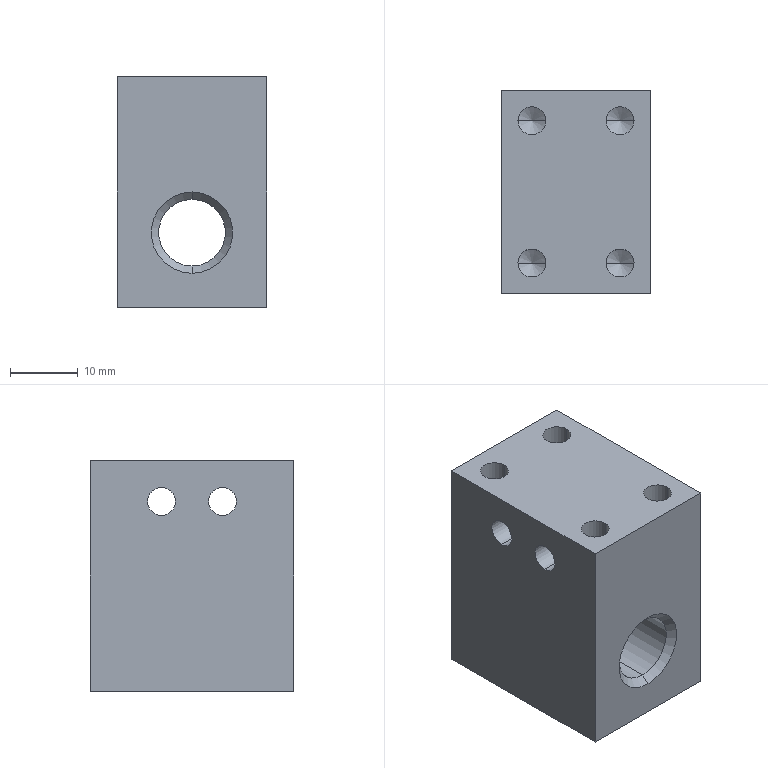Part | SolidWorks | features BaseBody 1 | 1 solid | 32 faces | box 22 x 30 x 34 mm | volume 18865 mm3 | cylinder 14 | cone 12 | plane 6 | commonest cylinder face diameters 4.134 x12 9.835 x2
STEP:
#1=CARTESIAN_POINT('',(279.547,1588.309,-1159.503));
#2=VERTEX_POINT('',#1);
#3=CARTESIAN_POINT('',(279.547,1588.309,-1163.637));
#4=VERTEX_POINT('',#3);
#5=CARTESIAN_POINT('',(279.547,1588.309,-1161.57));
#6=DIRECTION('',(1.,0.,0.));
#7=DIRECTION('',(0.,0.,-1.));
#8=AXIS2_PLACEMENT_3D('',#5,#6,#7);
#9=CIRCLE('',#8,2.067);
#10=EDGE_CURVE('',#2,#4,#9,.T.);
#11=ORIENTED_EDGE('',*,*,#10,.F.);
#12=CARTESIAN_POINT('',(301.547,1588.309,-1159.503));
#13=VERTEX_POINT('',#12);
#14=CARTESIAN_POINT('',(301.547,1588.309,-1159.503));
#15=DIRECTION('',(1.,0.,0.));
#16=VECTOR('',#15,1000.);
#17=LINE('',#14,#16);
#18=EDGE_CURVE('',#2,#13,#17,.T.);
#19=ORIENTED_EDGE('',*,*,#18,.T.);
#20=CARTESIAN_POINT('',(301.547,1588.309,-1163.637));
#21=VERTEX_POINT('',#20);
#22=CARTESIAN_POINT('',(301.547,1588.309,-1161.57));
#23=DIRECTION('',(1.,0.,0.));
#24=DIRECTION('',(0.,0.,-1.));
#25=AXIS2_PLACEMENT_3D('',#22,#23,#24);
#26=CIRCLE('',#25,2.067);
#27=EDGE_CURVE('',#13,#21,#26,.T.);
#28=ORIENTED_EDGE('',*,*,#27,.T.);
#29=CARTESIAN_POINT('',(301.547,1588.309,-1163.637));
#30=DIRECTION('',(1.,0.,0.));
#31=VECTOR('',#30,1000.);
#32=LINE('',#29,#31);
#33=EDGE_CURVE('',#4,#21,#32,.T.);
#34=ORIENTED_EDGE('',*,*,#33,.F.);
#35=EDGE_LOOP('',(#11,#19,#28,#34));
#36=FACE_OUTER_BOUND('',#35,.T.);
#37=CARTESIAN_POINT('',(301.547,1588.309,-1161.57));
#38=DIRECTION('',(1.,0.,0.));
#39=DIRECTION('',(0.,0.,-1.));
#40=AXIS2_PLACEMENT_3D('',#37,#38,#39);
#41=CYLINDRICAL_SURFACE('',#40,2.067);
#42=ADVANCED_FACE('',(#36),#41,.F.);
#43=CARTESIAN_POINT('',(279.547,1597.309,-1159.503));
#44=VERTEX_POINT('',#43);
#45=CARTESIAN_POINT('',(279.547,1597.309,-1163.637));
#46=VERTEX_POINT('',#45);
#47=CARTESIAN_POINT('',(279.547,1597.309,-1161.57));
#48=DIRECTION('',(1.,0.,0.));
#49=DIRECTION('',(0.,0.,-1.));
#50=AXIS2_PLACEMENT_3D('',#47,#48,#49);
#51=CIRCLE('',#50,2.067);
#52=EDGE_CURVE('',#44,#46,#51,.T.);
#53=ORIENTED_EDGE('',*,*,#52,.F.);
#54=CARTESIAN_POINT('',(301.547,1597.309,-1159.503));
#55=VERTEX_POINT('',#54);
#56=CARTESIAN_POINT('',(301.547,1597.309,-1159.503));
#57=DIRECTION('',(1.,0.,0.));
#58=VECTOR('',#57,1000.);
#59=LINE('',#56,#58);
#60=EDGE_CURVE('',#44,#55,#59,.T.);
#61=ORIENTED_EDGE('',*,*,#60,.T.);
#62=CARTESIAN_POINT('',(301.547,1597.309,-1163.637));
#63=VERTEX_POINT('',#62);
#64=CARTESIAN_POINT('',(301.547,1597.309,-1161.57));
#65=DIRECTION('',(1.,0.,0.));
#66=DIRECTION('',(0.,0.,-1.));
#67=AXIS2_PLACEMENT_3D('',#64,#65,#66);
#68=CIRCLE('',#67,2.067);
#69=EDGE_CURVE('',#55,#63,#68,.T.);
#70=ORIENTED_EDGE('',*,*,#69,.T.);
#71=CARTESIAN_POINT('',(301.547,1597.309,-1163.637));
#72=DIRECTION('',(1.,0.,0.));
#73=VECTOR('',#72,1000.);
#74=LINE('',#71,#73);
#75=EDGE_CURVE('',#46,#63,#74,.T.);
#76=ORIENTED_EDGE('',*,*,#75,.F.);
#77=EDGE_LOOP('',(#53,#61,#70,#76));
#78=FACE_OUTER_BOUND('',#77,.T.);
#79=CARTESIAN_POINT('',(301.547,1597.309,-1161.57));
#80=DIRECTION('',(1.,0.,0.));
#81=DIRECTION('',(0.,0.,-1.));
#82=AXIS2_PLACEMENT_3D('',#79,#80,#81);
#83=CYLINDRICAL_SURFACE('',#82,2.067);
#84=ADVANCED_FACE('',(#78),#83,.F.);
#85=CARTESIAN_POINT('',(290.547,1606.726,-1183.488));
#86=VERTEX_POINT('',#85);
#87=CARTESIAN_POINT('',(290.547,1606.726,-1173.652));
#88=VERTEX_POINT('',#87);
#89=CARTESIAN_POINT('',(290.547,1606.726,-1178.57));
#90=DIRECTION('',(0.,1.,0.));
#91=DIRECTION('',(-1.,0.,0.));
#92=AXIS2_PLACEMENT_3D('',#89,#90,#91);
#93=CIRCLE('',#92,4.918);
#94=EDGE_CURVE('',#86,#88,#93,.T.);
#95=ORIENTED_EDGE('',*,*,#94,.F.);
#96=CARTESIAN_POINT('',(290.547,1607.809,-1184.57));
#97=VERTEX_POINT('',#96);
#98=CARTESIAN_POINT('',(290.547,1607.809,-1184.57));
#99=DIRECTION('',(0.,0.7071,-0.7071));
#100=VECTOR('',#99,1000.);
#101=LINE('',#98,#100);
#102=EDGE_CURVE('',#86,#97,#101,.T.);
#103=ORIENTED_EDGE('',*,*,#102,.T.);
#104=CARTESIAN_POINT('',(290.547,1607.809,-1172.57));
#105=VERTEX_POINT('',#104);
#106=CARTESIAN_POINT('',(290.547,1607.809,-1178.57));
#107=DIRECTION('',(0.,-1.,0.));
#108=DIRECTION('',(0.,0.,1.));
#109=AXIS2_PLACEMENT_3D('',#106,#107,#108);
#110=CIRCLE('',#109,6.);
#111=EDGE_CURVE('',#105,#97,#110,.T.);
#112=ORIENTED_EDGE('',*,*,#111,.F.);
#113=CARTESIAN_POINT('',(290.547,1607.809,-1172.57));
#114=DIRECTION('',(0.,0.7071,0.7071));
#115=VECTOR('',#114,1000.);
#116=LINE('',#113,#115);
#117=EDGE_CURVE('',#88,#105,#116,.T.);
#118=ORIENTED_EDGE('',*,*,#117,.F.);
#119=EDGE_LOOP('',(#95,#103,#112,#118));
#120=FACE_OUTER_BOUND('',#119,.T.);
#121=CARTESIAN_POINT('',(290.547,1607.809,-1178.57));
#122=DIRECTION('',(0.,1.,0.));
#123=DIRECTION('',(0.,0.,1.));
#124=AXIS2_PLACEMENT_3D('',#121,#122,#123);
#125=CONICAL_SURFACE('',#124,6.,0.7854);
#126=ADVANCED_FACE('',(#120),#125,.F.);
#127=CARTESIAN_POINT('',(281.98,1603.309,-1167.57));
#128=VERTEX_POINT('',#127);
#129=CARTESIAN_POINT('',(286.114,1603.309,-1167.57));
#130=VERTEX_POINT('',#129);
#131=CARTESIAN_POINT('',(284.047,1603.309,-1167.57));
#132=DIRECTION('',(0.,0.,1.));
#133=DIRECTION('',(1.,0.,0.));
#134=AXIS2_PLACEMENT_3D('',#131,#132,#133);
#135=CIRCLE('',#134,2.067);
#136=EDGE_CURVE('',#128,#130,#135,.T.);
#137=ORIENTED_EDGE('',*,*,#136,.F.);
#138=CARTESIAN_POINT('',(281.98,1603.309,-1155.57));
#139=VERTEX_POINT('',#138);
#140=CARTESIAN_POINT('',(281.98,1603.309,-1155.57));
#141=DIRECTION('',(0.,0.,1.));
#142=VECTOR('',#141,1000.);
#143=LINE('',#140,#142);
#144=EDGE_CURVE('',#128,#139,#143,.T.);
#145=ORIENTED_EDGE('',*,*,#144,.T.);
#146=CARTESIAN_POINT('',(286.114,1603.309,-1155.57));
#147=VERTEX_POINT('',#146);
#148=CARTESIAN_POINT('',(284.047,1603.309,-1155.57));
#149=DIRECTION('',(0.,0.,1.));
#150=DIRECTION('',(1.,0.,0.));
#151=AXIS2_PLACEMENT_3D('',#148,#149,#150);
#152=CIRCLE('',#151,2.067);
#153=EDGE_CURVE('',#139,#147,#152,.T.);
#154=ORIENTED_EDGE('',*,*,#153,.T.);
#155=CARTESIAN_POINT('',(286.114,1603.309,-1155.57));
#156=DIRECTION('',(0.,0.,1.));
#157=VECTOR('',#156,1000.);
#158=LINE('',#155,#157);
#159=EDGE_CURVE('',#130,#147,#158,.T.);
#160=ORIENTED_EDGE('',*,*,#159,.F.);
#161=EDGE_LOOP('',(#137,#145,#154,#160));
#162=FACE_OUTER_BOUND('',#161,.T.);
#163=CARTESIAN_POINT('',(284.047,1603.309,-1155.57));
#164=DIRECTION('',(0.,0.,1.));
#165=DIRECTION('',(1.,0.,0.));
#166=AXIS2_PLACEMENT_3D('',#163,#164,#165);
#167=CYLINDRICAL_SURFACE('',#166,2.067);
#168=ADVANCED_FACE('',(#162),#167,.F.);
#169=CARTESIAN_POINT('',(294.98,1603.309,-1167.57));
#170=VERTEX_POINT('',#169);
#171=CARTESIAN_POINT('',(299.114,1603.309,-1167.57));
#172=VERTEX_POINT('',#171);
#173=CARTESIAN_POINT('',(297.047,1603.309,-1167.57));
#174=DIRECTION('',(0.,0.,1.));
#175=DIRECTION('',(1.,0.,0.));
#176=AXIS2_PLACEMENT_3D('',#173,#174,#175);
#177=CIRCLE('',#176,2.067);
#178=EDGE_CURVE('',#170,#172,#177,.T.);
#179=ORIENTED_EDGE('',*,*,#178,.F.);
#180=CARTESIAN_POINT('',(294.98,1603.309,-1155.57));
#181=VERTEX_POINT('',#180);
#182=CARTESIAN_POINT('',(294.98,1603.309,-1155.57));
#183=DIRECTION('',(0.,0.,1.));
#184=VECTOR('',#183,1000.);
#185=LINE('',#182,#184);
#186=EDGE_CURVE('',#170,#181,#185,.T.);
#187=ORIENTED_EDGE('',*,*,#186,.T.);
#188=CARTESIAN_POINT('',(299.114,1603.309,-1155.57));
#189=VERTEX_POINT('',#188);
#190=CARTESIAN_POINT('',(297.047,1603.309,-1155.57));
#191=DIRECTION('',(0.,0.,1.));
#192=DIRECTION('',(1.,0.,0.));
#193=AXIS2_PLACEMENT_3D('',#190,#191,#192);
#194=CIRCLE('',#193,2.067);
#195=EDGE_CURVE('',#181,#189,#194,.T.);
#196=ORIENTED_EDGE('',*,*,#195,.T.);
#197=CARTESIAN_POINT('',(299.114,1603.309,-1155.57));
#198=DIRECTION('',(0.,0.,1.));
#199=VECTOR('',#198,1000.);
#200=LINE('',#197,#199);
#201=EDGE_CURVE('',#172,#189,#200,.T.);
#202=ORIENTED_EDGE('',*,*,#201,.F.);
#203=EDGE_LOOP('',(#179,#187,#196,#202));
#204=FACE_OUTER_BOUND('',#203,.T.);
#205=CARTESIAN_POINT('',(297.047,1603.309,-1155.57));
#206=DIRECTION('',(0.,0.,1.));
#207=DIRECTION('',(1.,0.,0.));
#208=AXIS2_PLACEMENT_3D('',#205,#206,#207);
#209=CYLINDRICAL_SURFACE('',#208,2.067);
#210=ADVANCED_FACE('',(#204),#209,.F.);
#211=CARTESIAN_POINT('',(294.98,1582.309,-1167.57));
#212=VERTEX_POINT('',#211);
#213=CARTESIAN_POINT('',(299.114,1582.309,-1167.57));
#214=VERTEX_POINT('',#213);
#215=CARTESIAN_POINT('',(297.047,1582.309,-1167.57));
#216=DIRECTION('',(0.,0.,1.));
#217=DIRECTION('',(1.,0.,0.));
#218=AXIS2_PLACEMENT_3D('',#215,#216,#217);
#219=CIRCLE('',#218,2.067);
#220=EDGE_CURVE('',#212,#214,#219,.T.);
#221=ORIENTED_EDGE('',*,*,#220,.F.);
#222=CARTESIAN_POINT('',(294.98,1582.309,-1155.57));
#223=VERTEX_POINT('',#222);
#224=CARTESIAN_POINT('',(294.98,1582.309,-1155.57));
#225=DIRECTION('',(0.,0.,1.));
#226=VECTOR('',#225,1000.);
#227=LINE('',#224,#226);
#228=EDGE_CURVE('',#212,#223,#227,.T.);
#229=ORIENTED_EDGE('',*,*,#228,.T.);
#230=CARTESIAN_POINT('',(299.114,1582.309,-1155.57));
#231=VERTEX_POINT('',#230);
#232=CARTESIAN_POINT('',(297.047,1582.309,-1155.57));
#233=DIRECTION('',(0.,0.,1.));
#234=DIRECTION('',(1.,0.,0.));
#235=AXIS2_PLACEMENT_3D('',#232,#233,#234);
#236=CIRCLE('',#235,2.067);
#237=EDGE_CURVE('',#223,#231,#236,.T.);
#238=ORIENTED_EDGE('',*,*,#237,.T.);
#239=CARTESIAN_POINT('',(299.114,1582.309,-1155.57));
#240=DIRECTION('',(0.,0.,1.));
#241=VECTOR('',#240,1000.);
#242=LINE('',#239,#241);
#243=EDGE_CURVE('',#214,#231,#242,.T.);
#244=ORIENTED_EDGE('',*,*,#243,.F.);
#245=EDGE_LOOP('',(#221,#229,#238,#244));
#246=FACE_OUTER_BOUND('',#245,.T.);
#247=CARTESIAN_POINT('',(297.047,1582.309,-1155.57));
#248=DIRECTION('',(0.,0.,1.));
#249=DIRECTION('',(1.,0.,0.));
#250=AXIS2_PLACEMENT_3D('',#247,#248,#249);
#251=CYLINDRICAL_SURFACE('',#250,2.067);
#252=ADVANCED_FACE('',(#246),#251,.F.);
#253=CARTESIAN_POINT('',(281.98,1582.309,-1167.57));
#254=VERTEX_POINT('',#253);
#255=CARTESIAN_POINT('',(286.114,1582.309,-1167.57));
#256=VERTEX_POINT('',#255);
#257=CARTESIAN_POINT('',(284.047,1582.309,-1167.57));
#258=DIRECTION('',(0.,0.,1.));
#259=DIRECTION('',(1.,0.,0.));
#260=AXIS2_PLACEMENT_3D('',#257,#258,#259);
#261=CIRCLE('',#260,2.067);
#262=EDGE_CURVE('',#254,#256,#261,.T.);
#263=ORIENTED_EDGE('',*,*,#262,.F.);
#264=CARTESIAN_POINT('',(281.98,1582.309,-1155.57));
#265=VERTEX_POINT('',#264);
#266=CARTESIAN_POINT('',(281.98,1582.309,-1155.57));
#267=DIRECTION('',(0.,0.,1.));
#268=VECTOR('',#267,1000.);
#269=LINE('',#266,#268);
#270=EDGE_CURVE('',#254,#265,#269,.T.);
#271=ORIENTED_EDGE('',*,*,#270,.T.);
#272=CARTESIAN_POINT('',(286.114,1582.309,-1155.57));
#273=VERTEX_POINT('',#272);
#274=CARTESIAN_POINT('',(284.047,1582.309,-1155.57));
#275=DIRECTION('',(0.,0.,1.));
#276=DIRECTION('',(1.,0.,0.));
#277=AXIS2_PLACEMENT_3D('',#274,#275,#276);
#278=CIRCLE('',#277,2.067);
#279=EDGE_CURVE('',#265,#273,#278,.T.);
#280=ORIENTED_EDGE('',*,*,#279,.T.);
#281=CARTESIAN_POINT('',(286.114,1582.309,-1155.57));
#282=DIRECTION('',(0.,0.,1.));
#283=VECTOR('',#282,1000.);
#284=LINE('',#281,#283);
#285=EDGE_CURVE('',#256,#273,#284,.T.);
#286=ORIENTED_EDGE('',*,*,#285,.F.);
#287=EDGE_LOOP('',(#263,#271,#280,#286));
#288=FACE_OUTER_BOUND('',#287,.T.);
#289=CARTESIAN_POINT('',(284.047,1582.309,-1155.57));
#290=DIRECTION('',(0.,0.,1.));
#291=DIRECTION('',(1.,0.,0.));
#292=AXIS2_PLACEMENT_3D('',#289,#290,#291);
#293=CYLINDRICAL_SURFACE('',#292,2.067);
#294=ADVANCED_FACE('',(#288),#293,.F.);
#295=CARTESIAN_POINT('',(290.547,1578.891,-1173.652));
#296=VERTEX_POINT('',#295);
#297=CARTESIAN_POINT('',(290.547,1578.891,-1183.488));
#298=VERTEX_POINT('',#297);
#299=CARTESIAN_POINT('',(290.547,1578.891,-1178.57));
#300=DIRECTION('',(0.,-1.,0.));
#301=DIRECTION('',(1.,0.,0.));
#302=AXIS2_PLACEMENT_3D('',#299,#300,#301);
#303=CIRCLE('',#302,4.918);
#304=EDGE_CURVE('',#296,#298,#303,.T.);
#305=ORIENTED_EDGE('',*,*,#304,.F.);
#306=CARTESIAN_POINT('',(290.547,1577.809,-1172.57));
#307=VERTEX_POINT('',#306);
#308=CARTESIAN_POINT('',(290.547,1577.809,-1172.57));
#309=DIRECTION('',(0.,-0.7071,0.7071));
#310=VECTOR('',#309,1000.);
#311=LINE('',#308,#310);
#312=EDGE_CURVE('',#296,#307,#311,.T.);
#313=ORIENTED_EDGE('',*,*,#312,.T.);
#314=CARTESIAN_POINT('',(290.547,1577.809,-1184.57));
#315=VERTEX_POINT('',#314);
#316=CARTESIAN_POINT('',(290.547,1577.809,-1178.57));
#317=DIRECTION('',(0.,-1.,0.));
#318=DIRECTION('',(0.,0.,-1.));
#319=AXIS2_PLACEMENT_3D('',#316,#317,#318);
#320=CIRCLE('',#319,6.);
#321=EDGE_CURVE('',#307,#315,#320,.T.);
#322=ORIENTED_EDGE('',*,*,#321,.T.);
#323=CARTESIAN_POINT('',(290.547,1577.809,-1184.57));
#324=DIRECTION('',(0.,-0.7071,-0.7071));
#325=VECTOR('',#324,1000.);
#326=LINE('',#323,#325);
#327=EDGE_CURVE('',#298,#315,#326,.T.);
#328=ORIENTED_EDGE('',*,*,#327,.F.);
#329=EDGE_LOOP('',(#305,#313,#322,#328));
#330=FACE_OUTER_BOUND('',#329,.T.);
#331=CARTESIAN_POINT('',(290.547,1577.809,-1178.57));
#332=DIRECTION('',(0.,-1.,0.));
#333=DIRECTION('',(0.,0.,-1.));
#334=AXIS2_PLACEMENT_3D('',#331,#332,#333);
#335=CONICAL_SURFACE('',#334,6.,0.7854);
#336=ADVANCED_FACE('',(#330),#335,.F.);
#337=ORIENTED_EDGE('',*,*,#304,.T.);
#338=CARTESIAN_POINT('',(290.547,1607.809,-1183.487));
#339=DIRECTION('',(0.,1.,0.));
#340=VECTOR('',#339,1000.);
#341=LINE('',#338,#340);
#342=EDGE_CURVE('',#298,#86,#341,.T.);
#343=ORIENTED_EDGE('',*,*,#342,.T.);
#344=ORIENTED_EDGE('',*,*,#94,.T.);
#345=CARTESIAN_POINT('',(290.547,1607.809,-1173.652));
#346=DIRECTION('',(0.,1.,0.));
#347=VECTOR('',#346,1000.);
#348=LINE('',#345,#347);
#349=EDGE_CURVE('',#296,#88,#348,.T.);
#350=ORIENTED_EDGE('',*,*,#349,.F.);
#351=EDGE_LOOP('',(#337,#343,#344,#350));
#352=FACE_OUTER_BOUND('',#351,.T.);
#353=CARTESIAN_POINT('',(290.547,1607.809,-1178.57));
#354=DIRECTION('',(0.,1.,0.));
#355=DIRECTION('',(0.,0.,1.));
#356=AXIS2_PLACEMENT_3D('',#353,#354,#355);
#357=CYLINDRICAL_SURFACE('',#356,4.917);
#358=ADVANCED_FACE('',(#352),#357,.F.);
#359=CARTESIAN_POINT('',(284.047,1603.309,-1168.812));
#360=VERTEX_POINT('',#359);
#361=CARTESIAN_POINT('',(286.114,1603.309,-1167.57));
#362=DIRECTION('',(0.8572,0.,0.515));
#363=VECTOR('',#362,1000.);
#364=LINE('',#361,#363);
#365=EDGE_CURVE('',#360,#130,#364,.T.);
#366=ORIENTED_EDGE('',*,*,#365,.F.);
#367=CARTESIAN_POINT('',(281.98,1603.309,-1167.57));
#368=DIRECTION('',(-0.8572,0.,0.515));
#369=VECTOR('',#368,1000.);
#370=LINE('',#367,#369);
#371=EDGE_CURVE('',#360,#128,#370,.T.);
#372=ORIENTED_EDGE('',*,*,#371,.T.);
#373=ORIENTED_EDGE('',*,*,#136,.T.);
#374=EDGE_LOOP('',(#366,#372,#373));
#375=FACE_OUTER_BOUND('',#374,.T.);
#376=CARTESIAN_POINT('',(284.047,1603.309,-1167.57));
#377=DIRECTION('',(0.,0.,1.));
#378=DIRECTION('',(1.,0.,0.));
#379=AXIS2_PLACEMENT_3D('',#376,#377,#378);
#380=CONICAL_SURFACE('',#379,2.067,1.03);
#381=ADVANCED_FACE('',(#375),#380,.F.);
#382=CARTESIAN_POINT('',(297.047,1603.309,-1168.812));
#383=VERTEX_POINT('',#382);
#384=CARTESIAN_POINT('',(299.114,1603.309,-1167.57));
#385=DIRECTION('',(0.8572,0.,0.515));
#386=VECTOR('',#385,1000.);
#387=LINE('',#384,#386);
#388=EDGE_CURVE('',#383,#172,#387,.T.);
#389=ORIENTED_EDGE('',*,*,#388,.F.);
#390=CARTESIAN_POINT('',(294.98,1603.309,-1167.57));
#391=DIRECTION('',(-0.8572,0.,0.515));
#392=VECTOR('',#391,1000.);
#393=LINE('',#390,#392);
#394=EDGE_CURVE('',#383,#170,#393,.T.);
#395=ORIENTED_EDGE('',*,*,#394,.T.);
#396=ORIENTED_EDGE('',*,*,#178,.T.);
#397=EDGE_LOOP('',(#389,#395,#396));
#398=FACE_OUTER_BOUND('',#397,.T.);
#399=CARTESIAN_POINT('',(297.047,1603.309,-1167.57));
#400=DIRECTION('',(0.,0.,1.));
#401=DIRECTION('',(1.,0.,0.));
#402=AXIS2_PLACEMENT_3D('',#399,#400,#401);
#403=CONICAL_SURFACE('',#402,2.067,1.03);
#404=ADVANCED_FACE('',(#398),#403,.F.);
#405=CARTESIAN_POINT('',(297.047,1582.309,-1168.812));
#406=VERTEX_POINT('',#405);
#407=CARTESIAN_POINT('',(299.114,1582.309,-1167.57));
#408=DIRECTION('',(0.8572,0.,0.515));
#409=VECTOR('',#408,1000.);
#410=LINE('',#407,#409);
#411=EDGE_CURVE('',#406,#214,#410,.T.);
#412=ORIENTED_EDGE('',*,*,#411,.F.);
#413=CARTESIAN_POINT('',(294.98,1582.309,-1167.57));
#414=DIRECTION('',(-0.8572,0.,0.515));
#415=VECTOR('',#414,1000.);
#416=LINE('',#413,#415);
#417=EDGE_CURVE('',#406,#212,#416,.T.);
#418=ORIENTED_EDGE('',*,*,#417,.T.);
#419=ORIENTED_EDGE('',*,*,#220,.T.);
#420=EDGE_LOOP('',(#412,#418,#419));
#421=FACE_OUTER_BOUND('',#420,.T.);
#422=CARTESIAN_POINT('',(297.047,1582.309,-1167.57));
#423=DIRECTION('',(0.,0.,1.));
#424=DIRECTION('',(1.,0.,0.));
#425=AXIS2_PLACEMENT_3D('',#422,#423,#424);
#426=CONICAL_SURFACE('',#425,2.067,1.03);
#427=ADVANCED_FACE('',(#421),#426,.F.);
#428=CARTESIAN_POINT('',(284.047,1582.309,-1168.812));
#429=VERTEX_POINT('',#428);
#430=CARTESIAN_POINT('',(286.114,1582.309,-1167.57));
#431=DIRECTION('',(0.8572,0.,0.515));
#432=VECTOR('',#431,1000.);
#433=LINE('',#430,#432);
#434=EDGE_CURVE('',#429,#256,#433,.T.);
#435=ORIENTED_EDGE('',*,*,#434,.F.);
#436=CARTESIAN_POINT('',(281.98,1582.309,-1167.57));
#437=DIRECTION('',(-0.8572,0.,0.515));
#438=VECTOR('',#437,1000.);
#439=LINE('',#436,#438);
#440=EDGE_CURVE('',#429,#254,#439,.T.);
#441=ORIENTED_EDGE('',*,*,#440,.T.);
#442=ORIENTED_EDGE('',*,*,#262,.T.);
#443=EDGE_LOOP('',(#435,#441,#442));
#444=FACE_OUTER_BOUND('',#443,.T.);
#445=CARTESIAN_POINT('',(284.047,1582.309,-1167.57));
#446=DIRECTION('',(0.,0.,1.));
#447=DIRECTION('',(1.,0.,0.));
#448=AXIS2_PLACEMENT_3D('',#445,#446,#447);
#449=CONICAL_SURFACE('',#448,2.067,1.03);
#450=ADVANCED_FACE('',(#444),#449,.F.);
#451=CARTESIAN_POINT('',(301.547,1588.309,-1161.57));
#452=DIRECTION('',(1.,0.,0.));
#453=DIRECTION('',(0.,0.,-1.));
#454=AXIS2_PLACEMENT_3D('',#451,#452,#453);
#455=CIRCLE('',#454,2.067);
#456=EDGE_CURVE('',#21,#13,#455,.T.);
#457=ORIENTED_EDGE('',*,*,#456,.F.);
#458=ORIENTED_EDGE('',*,*,#27,.F.);
#459=EDGE_LOOP('',(#457,#458));
#460=FACE_BOUND('',#459,.T.);
#461=CARTESIAN_POINT('',(301.547,1597.309,-1161.57));
#462=DIRECTION('',(1.,0.,0.));
#463=DIRECTION('',(0.,0.,-1.));
#464=AXIS2_PLACEMENT_3D('',#461,#462,#463);
#465=CIRCLE('',#464,2.067);
#466=EDGE_CURVE('',#63,#55,#465,.T.);
#467=ORIENTED_EDGE('',*,*,#466,.F.);
#468=ORIENTED_EDGE('',*,*,#69,.F.);
#469=EDGE_LOOP('',(#467,#468));
#470=FACE_BOUND('',#469,.T.);
#471=CARTESIAN_POINT('',(301.547,1607.809,-1155.57));
#472=VERTEX_POINT('',#471);
#473=CARTESIAN_POINT('',(301.547,1607.809,-1189.57));
#474=VERTEX_POINT('',#473);
#475=CARTESIAN_POINT('',(301.547,1607.809,-1155.57));
#476=DIRECTION('',(0.,0.,-1.));
#477=VECTOR('',#476,1000.);
#478=LINE('',#475,#477);
#479=EDGE_CURVE('',#472,#474,#478,.T.);
#480=ORIENTED_EDGE('',*,*,#479,.F.);
#481=CARTESIAN_POINT('',(301.547,1577.809,-1155.57));
#482=VERTEX_POINT('',#481);
#483=CARTESIAN_POINT('',(301.547,1607.809,-1155.57));
#484=DIRECTION('',(0.,1.,0.));
#485=VECTOR('',#484,1000.);
#486=LINE('',#483,#485);
#487=EDGE_CURVE('',#482,#472,#486,.T.);
#488=ORIENTED_EDGE('',*,*,#487,.F.);
#489=CARTESIAN_POINT('',(301.547,1577.809,-1189.57));
#490=VERTEX_POINT('',#489);
#491=CARTESIAN_POINT('',(301.547,1577.809,-1155.57));
#492=DIRECTION('',(0.,0.,1.));
#493=VECTOR('',#492,1000.);
#494=LINE('',#491,#493);
#495=EDGE_CURVE('',#490,#482,#494,.T.);
#496=ORIENTED_EDGE('',*,*,#495,.F.);
#497=CARTESIAN_POINT('',(301.547,1607.809,-1189.57));
#498=DIRECTION('',(0.,-1.,0.));
#499=VECTOR('',#498,1000.);
#500=LINE('',#497,#499);
#501=EDGE_CURVE('',#474,#490,#500,.T.);
#502=ORIENTED_EDGE('',*,*,#501,.F.);
#503=EDGE_LOOP('',(#480,#488,#496,#502));
#504=FACE_OUTER_BOUND('',#503,.T.);
#505=CARTESIAN_POINT('',(301.547,1607.809,-1155.57));
#506=DIRECTION('',(-1.,0.,0.));
#507=DIRECTION('',(0.,0.,1.));
#508=AXIS2_PLACEMENT_3D('',#505,#506,#507);
#509=PLANE('',#508);
#510=ADVANCED_FACE('',(#460,#470,#504),#509,.F.);
#511=ORIENTED_EDGE('',*,*,#18,.F.);
#512=CARTESIAN_POINT('',(279.547,1588.309,-1161.57));
#513=DIRECTION('',(1.,0.,0.));
#514=DIRECTION('',(0.,0.,-1.));
#515=AXIS2_PLACEMENT_3D('',#512,#513,#514);
#516=CIRCLE('',#515,2.067);
#517=EDGE_CURVE('',#4,#2,#516,.T.);
#518=ORIENTED_EDGE('',*,*,#517,.F.);
#519=ORIENTED_EDGE('',*,*,#33,.T.);
#520=ORIENTED_EDGE('',*,*,#456,.T.);
#521=EDGE_LOOP('',(#511,#518,#519,#520));
#522=FACE_OUTER_BOUND('',#521,.T.);
#523=CARTESIAN_POINT('',(301.547,1588.309,-1161.57));
#524=DIRECTION('',(1.,0.,0.));
#525=DIRECTION('',(0.,0.,-1.));
#526=AXIS2_PLACEMENT_3D('',#523,#524,#525);
#527=CYLINDRICAL_SURFACE('',#526,2.067);
#528=ADVANCED_FACE('',(#522),#527,.F.);
#529=ORIENTED_EDGE('',*,*,#60,.F.);
#530=CARTESIAN_POINT('',(279.547,1597.309,-1161.57));
#531=DIRECTION('',(1.,0.,0.));
#532=DIRECTION('',(0.,0.,-1.));
#533=AXIS2_PLACEMENT_3D('',#530,#531,#532);
#534=CIRCLE('',#533,2.067);
#535=EDGE_CURVE('',#46,#44,#534,.T.);
#536=ORIENTED_EDGE('',*,*,#535,.F.);
#537=ORIENTED_EDGE('',*,*,#75,.T.);
#538=ORIENTED_EDGE('',*,*,#466,.T.);
#539=EDGE_LOOP('',(#529,#536,#537,#538));
#540=FACE_OUTER_BOUND('',#539,.T.);
#541=CARTESIAN_POINT('',(301.547,1597.309,-1161.57));
#542=DIRECTION('',(1.,0.,0.));
#543=DIRECTION('',(0.,0.,-1.));
#544=AXIS2_PLACEMENT_3D('',#541,#542,#543);
#545=CYLINDRICAL_SURFACE('',#544,2.067);
#546=ADVANCED_FACE('',(#540),#545,.F.);
#547=CARTESIAN_POINT('',(279.547,1607.809,-1189.57));
#548=VERTEX_POINT('',#547);
#549=CARTESIAN_POINT('',(301.547,1607.809,-1189.57));
#550=DIRECTION('',(-1.,0.,0.));
#551=VECTOR('',#550,1000.);
#552=LINE('',#549,#551);
#553=EDGE_CURVE('',#474,#548,#552,.T.);
#554=ORIENTED_EDGE('',*,*,#553,.F.);
#555=ORIENTED_EDGE('',*,*,#501,.T.);
#556=CARTESIAN_POINT('',(279.547,1577.809,-1189.57));
#557=VERTEX_POINT('',#556);
#558=CARTESIAN_POINT('',(301.547,1577.809,-1189.57));
#559=DIRECTION('',(1.,0.,0.));
#560=VECTOR('',#559,1000.);
#561=LINE('',#558,#560);
#562=EDGE_CURVE('',#557,#490,#561,.T.);
#563=ORIENTED_EDGE('',*,*,#562,.F.);
#564=CARTESIAN_POINT('',(279.547,1607.809,-1189.57));
#565=DIRECTION('',(0.,-1.,0.));
#566=VECTOR('',#565,1000.);
#567=LINE('',#564,#566);
#568=EDGE_CURVE('',#548,#557,#567,.T.);
#569=ORIENTED_EDGE('',*,*,#568,.F.);
#570=EDGE_LOOP('',(#554,#555,#563,#569));
#571=FACE_OUTER_BOUND('',#570,.T.);
#572=CARTESIAN_POINT('',(301.547,1607.809,-1189.57));
#573=DIRECTION('',(0.,0.,1.));
#574=DIRECTION('',(1.,0.,0.));
#575=AXIS2_PLACEMENT_3D('',#572,#573,#574);
#576=PLANE('',#575);
#577=ADVANCED_FACE('',(#571),#576,.F.);
#578=ORIENTED_EDGE('',*,*,#111,.T.);
#579=CARTESIAN_POINT('',(290.547,1607.809,-1178.57));
#580=DIRECTION('',(0.,-1.,0.));
#581=DIRECTION('',(0.,0.,1.));
#582=AXIS2_PLACEMENT_3D('',#579,#580,#581);
#583=CIRCLE('',#582,6.);
#584=EDGE_CURVE('',#97,#105,#583,.T.);
#585=ORIENTED_EDGE('',*,*,#584,.T.);
#586=EDGE_LOOP('',(#578,#585));
#587=FACE_BOUND('',#586,.T.);
#588=CARTESIAN_POINT('',(279.547,1607.809,-1155.57));
#589=VERTEX_POINT('',#588);
#590=CARTESIAN_POINT('',(290.547,1607.809,-1155.57));
#591=DIRECTION('',(1.,0.,0.));
#592=VECTOR('',#591,1000.);
#593=LINE('',#590,#592);
#594=EDGE_CURVE('',#589,#472,#593,.T.);
#595=ORIENTED_EDGE('',*,*,#594,.T.);
#596=ORIENTED_EDGE('',*,*,#479,.T.);
#597=ORIENTED_EDGE('',*,*,#553,.T.);
#598=CARTESIAN_POINT('',(279.547,1607.809,-1155.57));
#599=DIRECTION('',(0.,0.,1.));
#600=VECTOR('',#599,1000.);
#601=LINE('',#598,#600);
#602=EDGE_CURVE('',#548,#589,#601,.T.);
#603=ORIENTED_EDGE('',*,*,#602,.T.);
#604=EDGE_LOOP('',(#595,#596,#597,#603));
#605=FACE_OUTER_BOUND('',#604,.T.);
#606=CARTESIAN_POINT('',(290.547,1607.809,-1155.57));
#607=DIRECTION('',(0.,1.,0.));
#608=DIRECTION('',(0.,0.,1.));
#609=AXIS2_PLACEMENT_3D('',#606,#607,#608);
#610=PLANE('',#609);
#611=ADVANCED_FACE('',(#587,#605),#610,.T.);
#612=CARTESIAN_POINT('',(284.047,1603.309,-1155.57));
#613=DIRECTION('',(0.,0.,1.));
#614=DIRECTION('',(1.,0.,0.));
#615=AXIS2_PLACEMENT_3D('',#612,#613,#614);
#616=CIRCLE('',#615,2.067);
#617=EDGE_CURVE('',#147,#139,#616,.T.);
#618=ORIENTED_EDGE('',*,*,#617,.F.);
#619=ORIENTED_EDGE('',*,*,#153,.F.);
#620=EDGE_LOOP('',(#618,#619));
#621=FACE_BOUND('',#620,.T.);
#622=CARTESIAN_POINT('',(297.047,1603.309,-1155.57));
#623=DIRECTION('',(0.,0.,1.));
#624=DIRECTION('',(1.,0.,0.));
#625=AXIS2_PLACEMENT_3D('',#622,#623,#624);
#626=CIRCLE('',#625,2.067);
#627=EDGE_CURVE('',#189,#181,#626,.T.);
#628=ORIENTED_EDGE('',*,*,#627,.F.);
#629=ORIENTED_EDGE('',*,*,#195,.F.);
#630=EDGE_LOOP('',(#628,#629));
#631=FACE_BOUND('',#630,.T.);
#632=CARTESIAN_POINT('',(297.047,1582.309,-1155.57));
#633=DIRECTION('',(0.,0.,1.));
#634=DIRECTION('',(1.,0.,0.));
#635=AXIS2_PLACEMENT_3D('',#632,#633,#634);
#636=CIRCLE('',#635,2.067);
#637=EDGE_CURVE('',#231,#223,#636,.T.);
#638=ORIENTED_EDGE('',*,*,#637,.F.);
#639=ORIENTED_EDGE('',*,*,#237,.F.);
#640=EDGE_LOOP('',(#638,#639));
#641=FACE_BOUND('',#640,.T.);
#642=CARTESIAN_POINT('',(284.047,1582.309,-1155.57));
#643=DIRECTION('',(0.,0.,1.));
#644=DIRECTION('',(1.,0.,0.));
#645=AXIS2_PLACEMENT_3D('',#642,#643,#644);
#646=CIRCLE('',#645,2.067);
#647=EDGE_CURVE('',#273,#265,#646,.T.);
#648=ORIENTED_EDGE('',*,*,#647,.F.);
#649=ORIENTED_EDGE('',*,*,#279,.F.);
#650=EDGE_LOOP('',(#648,#649));
#651=FACE_BOUND('',#650,.T.);
#652=ORIENTED_EDGE('',*,*,#594,.F.);
#653=CARTESIAN_POINT('',(279.547,1577.809,-1155.57));
#654=VERTEX_POINT('',#653);
#655=CARTESIAN_POINT('',(279.547,1607.809,-1155.57));
#656=DIRECTION('',(0.,1.,0.));
#657=VECTOR('',#656,1000.);
#658=LINE('',#655,#657);
#659=EDGE_CURVE('',#654,#589,#658,.T.);
#660=ORIENTED_EDGE('',*,*,#659,.F.);
#661=CARTESIAN_POINT('',(301.547,1577.809,-1155.57));
#662=DIRECTION('',(-1.,0.,0.));
#663=VECTOR('',#662,1000.);
#664=LINE('',#661,#663);
#665=EDGE_CURVE('',#482,#654,#664,.T.);
#666=ORIENTED_EDGE('',*,*,#665,.F.);
#667=ORIENTED_EDGE('',*,*,#487,.T.);
#668=EDGE_LOOP('',(#652,#660,#666,#667));
#669=FACE_OUTER_BOUND('',#668,.T.);
#670=CARTESIAN_POINT('',(301.547,1607.809,-1155.57));
#671=DIRECTION('',(0.,0.,-1.));
#672=DIRECTION('',(-1.,0.,0.));
#673=AXIS2_PLACEMENT_3D('',#670,#671,#672);
#674=PLANE('',#673);
#675=ADVANCED_FACE('',(#621,#631,#641,#651,#669),#674,.F.);
#676=CARTESIAN_POINT('',(290.547,1577.809,-1178.57));
#677=DIRECTION('',(0.,-1.,0.));
#678=DIRECTION('',(0.,0.,-1.));
#679=AXIS2_PLACEMENT_3D('',#676,#677,#678);
#680=CIRCLE('',#679,6.);
#681=EDGE_CURVE('',#315,#307,#680,.T.);
#682=ORIENTED_EDGE('',*,*,#681,.F.);
#683=ORIENTED_EDGE('',*,*,#321,.F.);
#684=EDGE_LOOP('',(#682,#683));
#685=FACE_BOUND('',#684,.T.);
#686=CARTESIAN_POINT('',(279.547,1577.809,-1155.57));
#687=DIRECTION('',(0.,0.,1.));
#688=VECTOR('',#687,1000.);
#689=LINE('',#686,#688);
#690=EDGE_CURVE('',#557,#654,#689,.T.);
#691=ORIENTED_EDGE('',*,*,#690,.F.);
#692=ORIENTED_EDGE('',*,*,#562,.T.);
#693=ORIENTED_EDGE('',*,*,#495,.T.);
#694=ORIENTED_EDGE('',*,*,#665,.T.);
#695=EDGE_LOOP('',(#691,#692,#693,#694));
#696=FACE_OUTER_BOUND('',#695,.T.);
#697=CARTESIAN_POINT('',(290.547,1577.809,-1155.57));
#698=DIRECTION('',(0.,1.,0.));
#699=DIRECTION('',(0.,0.,1.));
#700=AXIS2_PLACEMENT_3D('',#697,#698,#699);
#701=PLANE('',#700);
#702=ADVANCED_FACE('',(#685,#696),#701,.F.);
#703=ORIENTED_EDGE('',*,*,#517,.T.);
#704=ORIENTED_EDGE('',*,*,#10,.T.);
#705=EDGE_LOOP('',(#703,#704));
#706=FACE_BOUND('',#705,.T.);
#707=ORIENTED_EDGE('',*,*,#535,.T.);
#708=ORIENTED_EDGE('',*,*,#52,.T.);
#709=EDGE_LOOP('',(#707,#708));
#710=FACE_BOUND('',#709,.T.);
#711=ORIENTED_EDGE('',*,*,#602,.F.);
#712=ORIENTED_EDGE('',*,*,#568,.T.);
#713=ORIENTED_EDGE('',*,*,#690,.T.);
#714=ORIENTED_EDGE('',*,*,#659,.T.);
#715=EDGE_LOOP('',(#711,#712,#713,#714));
#716=FACE_OUTER_BOUND('',#715,.T.);
#717=CARTESIAN_POINT('',(279.547,1607.809,-1155.57));
#718=DIRECTION('',(1.,0.,0.));
#719=DIRECTION('',(0.,0.,-1.));
#720=AXIS2_PLACEMENT_3D('',#717,#718,#719);
#721=PLANE('',#720);
#722=ADVANCED_FACE('',(#706,#710,#716),#721,.F.);
#723=ORIENTED_EDGE('',*,*,#102,.F.);
#724=CARTESIAN_POINT('',(290.547,1606.726,-1178.57));
#725=DIRECTION('',(0.,1.,0.));
#726=DIRECTION('',(-1.,0.,0.));
#727=AXIS2_PLACEMENT_3D('',#724,#725,#726);
#728=CIRCLE('',#727,4.918);
#729=EDGE_CURVE('',#88,#86,#728,.T.);
#730=ORIENTED_EDGE('',*,*,#729,.F.);
#731=ORIENTED_EDGE('',*,*,#117,.T.);
#732=ORIENTED_EDGE('',*,*,#584,.F.);
#733=EDGE_LOOP('',(#723,#730,#731,#732));
#734=FACE_OUTER_BOUND('',#733,.T.);
#735=CARTESIAN_POINT('',(290.547,1607.809,-1178.57));
#736=DIRECTION('',(0.,1.,0.));
#737=DIRECTION('',(0.,0.,1.));
#738=AXIS2_PLACEMENT_3D('',#735,#736,#737);
#739=CONICAL_SURFACE('',#738,6.,0.7854);
#740=ADVANCED_FACE('',(#734),#739,.F.);
#741=ORIENTED_EDGE('',*,*,#144,.F.);
#742=CARTESIAN_POINT('',(284.047,1603.309,-1167.57));
#743=DIRECTION('',(0.,0.,1.));
#744=DIRECTION('',(1.,0.,0.));
#745=AXIS2_PLACEMENT_3D('',#742,#743,#744);
#746=CIRCLE('',#745,2.067);
#747=EDGE_CURVE('',#130,#128,#746,.T.);
#748=ORIENTED_EDGE('',*,*,#747,.F.);
#749=ORIENTED_EDGE('',*,*,#159,.T.);
#750=ORIENTED_EDGE('',*,*,#617,.T.);
#751=EDGE_LOOP('',(#741,#748,#749,#750));
#752=FACE_OUTER_BOUND('',#751,.T.);
#753=CARTESIAN_POINT('',(284.047,1603.309,-1155.57));
#754=DIRECTION('',(0.,0.,1.));
#755=DIRECTION('',(1.,0.,0.));
#756=AXIS2_PLACEMENT_3D('',#753,#754,#755);
#757=CYLINDRICAL_SURFACE('',#756,2.067);
#758=ADVANCED_FACE('',(#752),#757,.F.);
#759=ORIENTED_EDGE('',*,*,#186,.F.);
#760=CARTESIAN_POINT('',(297.047,1603.309,-1167.57));
#761=DIRECTION('',(0.,0.,1.));
#762=DIRECTION('',(1.,0.,0.));
#763=AXIS2_PLACEMENT_3D('',#760,#761,#762);
#764=CIRCLE('',#763,2.067);
#765=EDGE_CURVE('',#172,#170,#764,.T.);
#766=ORIENTED_EDGE('',*,*,#765,.F.);
#767=ORIENTED_EDGE('',*,*,#201,.T.);
#768=ORIENTED_EDGE('',*,*,#627,.T.);
#769=EDGE_LOOP('',(#759,#766,#767,#768));
#770=FACE_OUTER_BOUND('',#769,.T.);
#771=CARTESIAN_POINT('',(297.047,1603.309,-1155.57));
#772=DIRECTION('',(0.,0.,1.));
#773=DIRECTION('',(1.,0.,0.));
#774=AXIS2_PLACEMENT_3D('',#771,#772,#773);
#775=CYLINDRICAL_SURFACE('',#774,2.067);
#776=ADVANCED_FACE('',(#770),#775,.F.);
#777=ORIENTED_EDGE('',*,*,#228,.F.);
#778=CARTESIAN_POINT('',(297.047,1582.309,-1167.57));
#779=DIRECTION('',(0.,0.,1.));
#780=DIRECTION('',(1.,0.,0.));
#781=AXIS2_PLACEMENT_3D('',#778,#779,#780);
#782=CIRCLE('',#781,2.067);
#783=EDGE_CURVE('',#214,#212,#782,.T.);
#784=ORIENTED_EDGE('',*,*,#783,.F.);
#785=ORIENTED_EDGE('',*,*,#243,.T.);
#786=ORIENTED_EDGE('',*,*,#637,.T.);
#787=EDGE_LOOP('',(#777,#784,#785,#786));
#788=FACE_OUTER_BOUND('',#787,.T.);
#789=CARTESIAN_POINT('',(297.047,1582.309,-1155.57));
#790=DIRECTION('',(0.,0.,1.));
#791=DIRECTION('',(1.,0.,0.));
#792=AXIS2_PLACEMENT_3D('',#789,#790,#791);
#793=CYLINDRICAL_SURFACE('',#792,2.067);
#794=ADVANCED_FACE('',(#788),#793,.F.);
#795=ORIENTED_EDGE('',*,*,#270,.F.);
#796=CARTESIAN_POINT('',(284.047,1582.309,-1167.57));
#797=DIRECTION('',(0.,0.,1.));
#798=DIRECTION('',(1.,0.,0.));
#799=AXIS2_PLACEMENT_3D('',#796,#797,#798);
#800=CIRCLE('',#799,2.067);
#801=EDGE_CURVE('',#256,#254,#800,.T.);
#802=ORIENTED_EDGE('',*,*,#801,.F.);
#803=ORIENTED_EDGE('',*,*,#285,.T.);
#804=ORIENTED_EDGE('',*,*,#647,.T.);
#805=EDGE_LOOP('',(#795,#802,#803,#804));
#806=FACE_OUTER_BOUND('',#805,.T.);
#807=CARTESIAN_POINT('',(284.047,1582.309,-1155.57));
#808=DIRECTION('',(0.,0.,1.));
#809=DIRECTION('',(1.,0.,0.));
#810=AXIS2_PLACEMENT_3D('',#807,#808,#809);
#811=CYLINDRICAL_SURFACE('',#810,2.067);
#812=ADVANCED_FACE('',(#806),#811,.F.);
#813=ORIENTED_EDGE('',*,*,#312,.F.);
#814=CARTESIAN_POINT('',(290.547,1578.891,-1178.57));
#815=DIRECTION('',(0.,-1.,0.));
#816=DIRECTION('',(1.,0.,0.));
#817=AXIS2_PLACEMENT_3D('',#814,#815,#816);
#818=CIRCLE('',#817,4.918);
#819=EDGE_CURVE('',#298,#296,#818,.T.);
#820=ORIENTED_EDGE('',*,*,#819,.F.);
#821=ORIENTED_EDGE('',*,*,#327,.T.);
#822=ORIENTED_EDGE('',*,*,#681,.T.);
#823=EDGE_LOOP('',(#813,#820,#821,#822));
#824=FACE_OUTER_BOUND('',#823,.T.);
#825=CARTESIAN_POINT('',(290.547,1577.809,-1178.57));
#826=DIRECTION('',(0.,-1.,0.));
#827=DIRECTION('',(0.,0.,-1.));
#828=AXIS2_PLACEMENT_3D('',#825,#826,#827);
#829=CONICAL_SURFACE('',#828,6.,0.7854);
#830=ADVANCED_FACE('',(#824),#829,.F.);
#831=ORIENTED_EDGE('',*,*,#342,.F.);
#832=ORIENTED_EDGE('',*,*,#819,.T.);
#833=ORIENTED_EDGE('',*,*,#349,.T.);
#834=ORIENTED_EDGE('',*,*,#729,.T.);
#835=EDGE_LOOP('',(#831,#832,#833,#834));
#836=FACE_OUTER_BOUND('',#835,.T.);
#837=CARTESIAN_POINT('',(290.547,1607.809,-1178.57));
#838=DIRECTION('',(0.,1.,0.));
#839=DIRECTION('',(0.,0.,1.));
#840=AXIS2_PLACEMENT_3D('',#837,#838,#839);
#841=CYLINDRICAL_SURFACE('',#840,4.917);
#842=ADVANCED_FACE('',(#836),#841,.F.);
#843=ORIENTED_EDGE('',*,*,#371,.F.);
#844=ORIENTED_EDGE('',*,*,#365,.T.);
#845=ORIENTED_EDGE('',*,*,#747,.T.);
#846=EDGE_LOOP('',(#843,#844,#845));
#847=FACE_OUTER_BOUND('',#846,.T.);
#848=CARTESIAN_POINT('',(284.047,1603.309,-1167.57));
#849=DIRECTION('',(0.,0.,1.));
#850=DIRECTION('',(1.,0.,0.));
#851=AXIS2_PLACEMENT_3D('',#848,#849,#850);
#852=CONICAL_SURFACE('',#851,2.067,1.03);
#853=ADVANCED_FACE('',(#847),#852,.F.);
#854=ORIENTED_EDGE('',*,*,#394,.F.);
#855=ORIENTED_EDGE('',*,*,#388,.T.);
#856=ORIENTED_EDGE('',*,*,#765,.T.);
#857=EDGE_LOOP('',(#854,#855,#856));
#858=FACE_OUTER_BOUND('',#857,.T.);
#859=CARTESIAN_POINT('',(297.047,1603.309,-1167.57));
#860=DIRECTION('',(0.,0.,1.));
#861=DIRECTION('',(1.,0.,0.));
#862=AXIS2_PLACEMENT_3D('',#859,#860,#861);
#863=CONICAL_SURFACE('',#862,2.067,1.03);
#864=ADVANCED_FACE('',(#858),#863,.F.);
#865=ORIENTED_EDGE('',*,*,#417,.F.);
#866=ORIENTED_EDGE('',*,*,#411,.T.);
#867=ORIENTED_EDGE('',*,*,#783,.T.);
#868=EDGE_LOOP('',(#865,#866,#867));
#869=FACE_OUTER_BOUND('',#868,.T.);
#870=CARTESIAN_POINT('',(297.047,1582.309,-1167.57));
#871=DIRECTION('',(0.,0.,1.));
#872=DIRECTION('',(1.,0.,0.));
#873=AXIS2_PLACEMENT_3D('',#870,#871,#872);
#874=CONICAL_SURFACE('',#873,2.067,1.03);
#875=ADVANCED_FACE('',(#869),#874,.F.);
#876=ORIENTED_EDGE('',*,*,#440,.F.);
#877=ORIENTED_EDGE('',*,*,#434,.T.);
#878=ORIENTED_EDGE('',*,*,#801,.T.);
#879=EDGE_LOOP('',(#876,#877,#878));
#880=FACE_OUTER_BOUND('',#879,.T.);
#881=CARTESIAN_POINT('',(284.047,1582.309,-1167.57));
#882=DIRECTION('',(0.,0.,1.));
#883=DIRECTION('',(1.,0.,0.));
#884=AXIS2_PLACEMENT_3D('',#881,#882,#883);
#885=CONICAL_SURFACE('',#884,2.067,1.03);
#886=ADVANCED_FACE('',(#880),#885,.F.);
#887=CLOSED_SHELL('',(#42,#84,#126,#168,#210,#252,#294,#336,#358,#381,#404,#427,#450,#510,#528,#546,#577,#611,#675,#702,#722,#740,#758,#776,#794,#812,#830,#842,#853,#864,#875,#886));
#888=MANIFOLD_SOLID_BREP('',#887);
#889=CARTESIAN_POINT('',(0.,0.,0.));
#890=DIRECTION('',(0.,0.,1.));
#891=DIRECTION('',(1.,0.,0.));
#892=AXIS2_PLACEMENT_3D('',#889,#890,#891);
#893=(LENGTH_UNIT()NAMED_UNIT(*)SI_UNIT(.MILLI.,.METRE.));
#894=UNCERTAINTY_MEASURE_WITH_UNIT(LENGTH_MEASURE(0.00001),#893,'','');
#895=(NAMED_UNIT(*)PLANE_ANGLE_UNIT()SI_UNIT($,.RADIAN.));
#896=(NAMED_UNIT(*)SI_UNIT($,.STERADIAN.)SOLID_ANGLE_UNIT());
#897=(GEOMETRIC_REPRESENTATION_CONTEXT(3)GLOBAL_UNCERTAINTY_ASSIGNED_CONTEXT((#894))GLOBAL_UNIT_ASSIGNED_CONTEXT((#893,#895,#896))REPRESENTATION_CONTEXT('',''));
#898=ADVANCED_BREP_SHAPE_REPRESENTATION('',(#888,#892),#897);